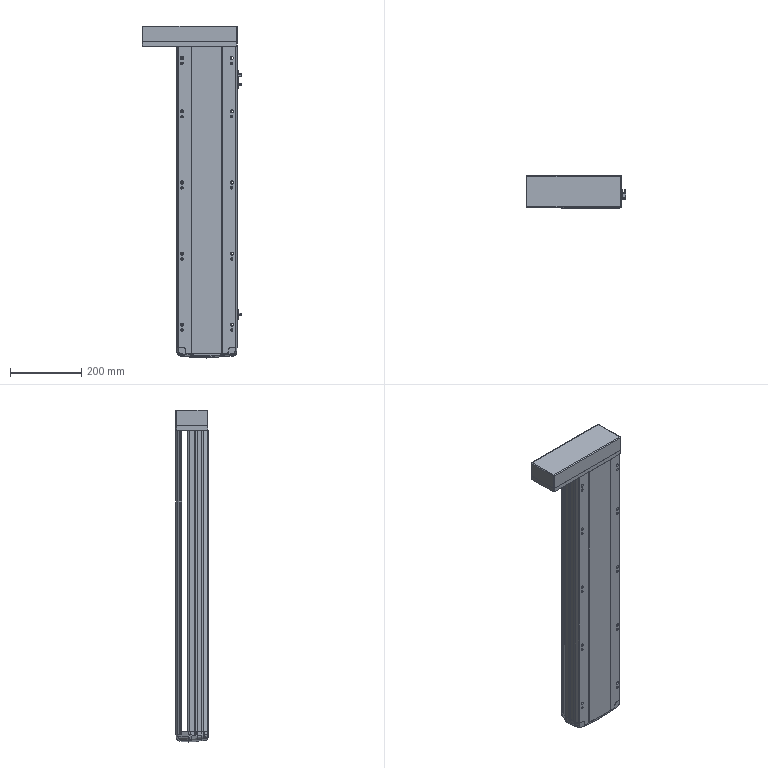Part | STEP file | Single-axis manipulator CFS17-L10-650-BR-T750-C4-MB-3M-body | 11 solids | 1331 faces | box 280.5 x 91 x 933.5 mm | volume 7444540 mm3 | plane 705 | cylinder 329 | spline 287 | other 10 | commonest cylinder face diameters 1 x46 0.6 x28 9 x28 1.5 x24 2 x22 6.8 x20